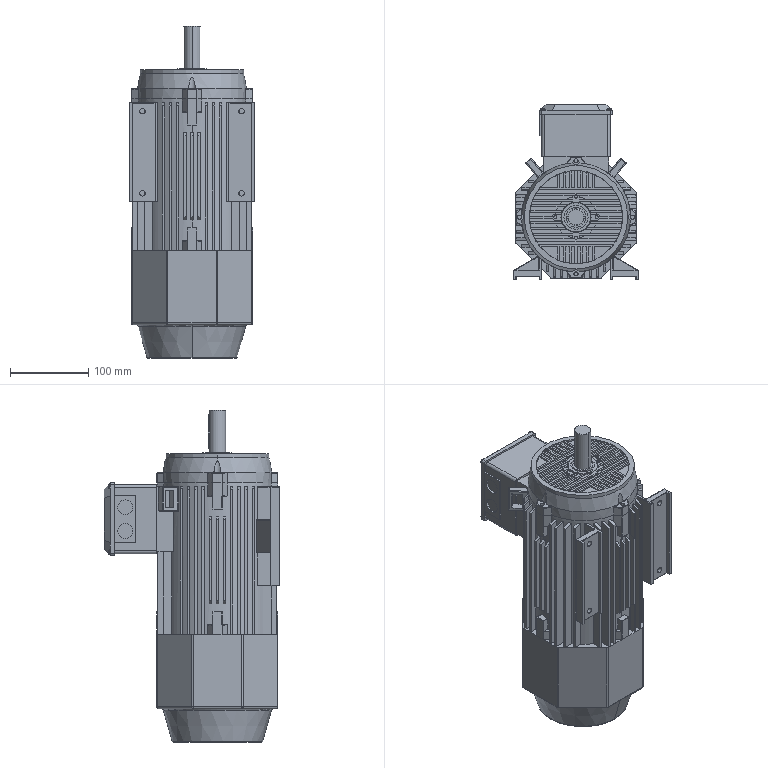Part | SolidWorks | features ICE 39, Fillet 12, MirrorPattern 12, CirPattern 5, LPattern 3, Revolution 3, Chamfer 1, Dome 1, Extrusion 1, LibraryFeature 1, PLine 1, RevCut 1, Scale 1 | 2 solids | 1414 faces | box 160 x 225 x 425 mm | volume 6896935 mm3 | plane 1010 | cylinder 298 | sphere 40 | cone 28 | torus 22 | spline 16 | commonest cylinder face diameters 1 x118 1.5 x22 2 x21 5 x20 92.628 x20 53.01 x16